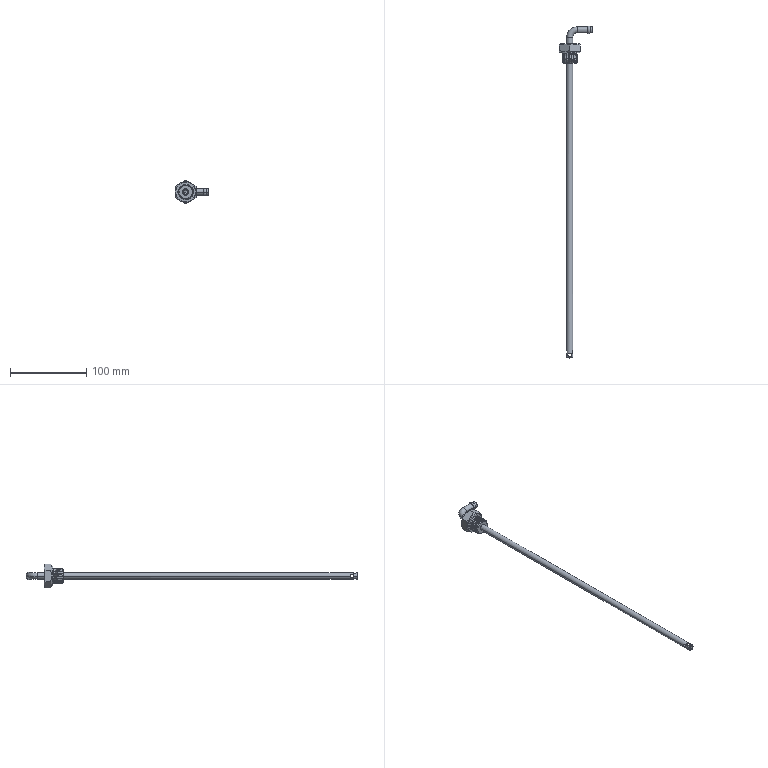Part | SolidWorks | features CompositeCurve 2 | 2 solids | 77 faces | box 43.501 x 435 x 31.18 mm | volume 19603 mm3 | cylinder 37 | torus 17 | plane 13 | cone 6 | spline 4 | commonest cylinder face diameters 20 x15 5 x8 8 x6 6 x4 8.5 x2 26 x2